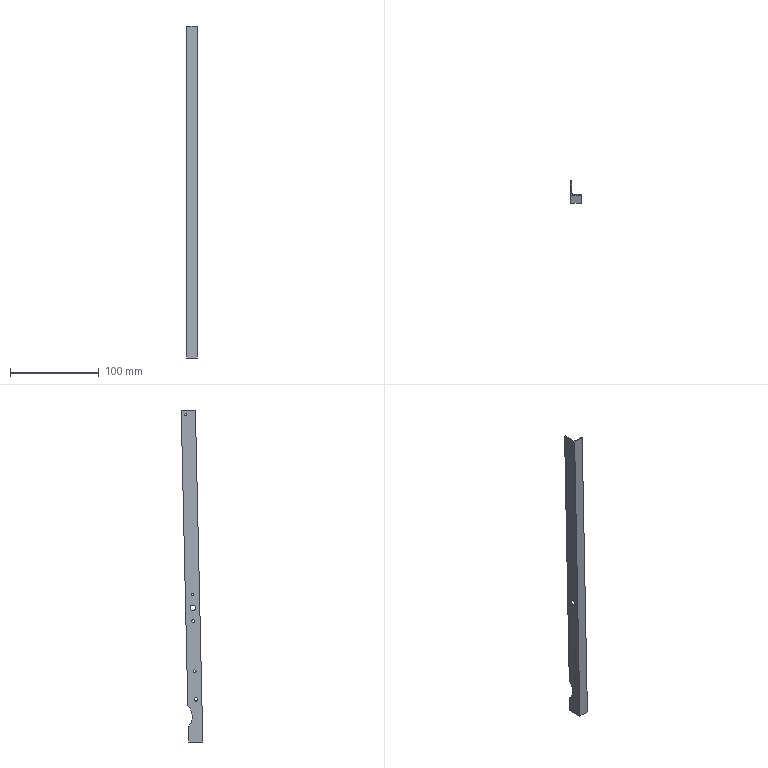Part | SolidWorks | features BaseBody 1 | 1 solid | 25 faces | box 12 x 24.318 x 374.05 mm | volume 11925 mm3 | cylinder 13 | plane 11 | spline 1 | commonest cylinder face diameters 3.2 x6 2.4 x2 4 x2 6.35 x2 36 x1
STEP:
#1=CARTESIAN_POINT('',(186.7,-128.619,106.65));
#2=VERTEX_POINT('',#1);
#3=CARTESIAN_POINT('',(186.7,-128.619,103.45));
#4=VERTEX_POINT('',#3);
#5=CARTESIAN_POINT('',(186.7,-128.619,105.05));
#6=DIRECTION('',(1.,0.,0.));
#7=DIRECTION('',(0.,0.,1.));
#8=AXIS2_PLACEMENT_3D('',#5,#6,#7);
#9=CIRCLE('',#8,1.6);
#10=EDGE_CURVE('',#2,#4,#9,.T.);
#11=ORIENTED_EDGE('',*,*,#10,.T.);
#12=CARTESIAN_POINT('',(185.5,-128.619,103.45));
#13=VERTEX_POINT('',#12);
#14=CARTESIAN_POINT('',(186.7,-128.619,103.45));
#15=DIRECTION('',(-1.,0.,0.));
#16=VECTOR('',#15,1000.);
#17=LINE('',#14,#16);
#18=EDGE_CURVE('',#4,#13,#17,.T.);
#19=ORIENTED_EDGE('',*,*,#18,.T.);
#20=CARTESIAN_POINT('',(185.5,-128.619,106.65));
#21=VERTEX_POINT('',#20);
#22=CARTESIAN_POINT('',(185.5,-128.619,105.05));
#23=DIRECTION('',(-1.,0.,0.));
#24=DIRECTION('',(0.,0.,1.));
#25=AXIS2_PLACEMENT_3D('',#22,#23,#24);
#26=CIRCLE('',#25,1.6);
#27=EDGE_CURVE('',#13,#21,#26,.T.);
#28=ORIENTED_EDGE('',*,*,#27,.T.);
#29=CARTESIAN_POINT('',(186.7,-128.619,106.65));
#30=DIRECTION('',(-1.,0.,0.));
#31=VECTOR('',#30,1000.);
#32=LINE('',#29,#31);
#33=EDGE_CURVE('',#2,#21,#32,.T.);
#34=ORIENTED_EDGE('',*,*,#33,.F.);
#35=EDGE_LOOP('',(#11,#19,#28,#34));
#36=FACE_OUTER_BOUND('',#35,.T.);
#37=CARTESIAN_POINT('',(186.7,-128.619,105.05));
#38=DIRECTION('',(-1.,0.,0.));
#39=DIRECTION('',(0.,0.,1.));
#40=AXIS2_PLACEMENT_3D('',#37,#38,#39);
#41=CYLINDRICAL_SURFACE('',#40,1.6);
#42=ADVANCED_FACE('',(#36),#41,.F.);
#43=CARTESIAN_POINT('',(185.5,-130.,71.45));
#44=VERTEX_POINT('',#43);
#45=CARTESIAN_POINT('',(185.5,-130.,75.45));
#46=VERTEX_POINT('',#45);
#47=CARTESIAN_POINT('',(185.5,-130.,73.45));
#48=DIRECTION('',(-1.,0.,0.));
#49=DIRECTION('',(0.,0.,-1.));
#50=AXIS2_PLACEMENT_3D('',#47,#48,#49);
#51=CIRCLE('',#50,2.);
#52=EDGE_CURVE('',#44,#46,#51,.T.);
#53=ORIENTED_EDGE('',*,*,#52,.T.);
#54=CARTESIAN_POINT('',(186.7,-130.,75.45));
#55=VERTEX_POINT('',#54);
#56=CARTESIAN_POINT('',(185.5,-130.,75.45));
#57=DIRECTION('',(1.,0.,0.));
#58=VECTOR('',#57,1000.);
#59=LINE('',#56,#58);
#60=EDGE_CURVE('',#46,#55,#59,.T.);
#61=ORIENTED_EDGE('',*,*,#60,.T.);
#62=CARTESIAN_POINT('',(186.7,-130.,71.45));
#63=VERTEX_POINT('',#62);
#64=CARTESIAN_POINT('',(186.7,-130.,73.45));
#65=DIRECTION('',(1.,0.,0.));
#66=DIRECTION('',(0.,0.,-1.));
#67=AXIS2_PLACEMENT_3D('',#64,#65,#66);
#68=CIRCLE('',#67,2.);
#69=EDGE_CURVE('',#55,#63,#68,.T.);
#70=ORIENTED_EDGE('',*,*,#69,.T.);
#71=CARTESIAN_POINT('',(185.5,-130.,71.45));
#72=DIRECTION('',(1.,0.,0.));
#73=VECTOR('',#72,1000.);
#74=LINE('',#71,#73);
#75=EDGE_CURVE('',#44,#63,#74,.T.);
#76=ORIENTED_EDGE('',*,*,#75,.F.);
#77=EDGE_LOOP('',(#53,#61,#70,#76));
#78=FACE_OUTER_BOUND('',#77,.T.);
#79=CARTESIAN_POINT('',(185.5,-130.,73.45));
#80=DIRECTION('',(1.,0.,0.));
#81=DIRECTION('',(0.,0.,-1.));
#82=AXIS2_PLACEMENT_3D('',#79,#80,#81);
#83=CYLINDRICAL_SURFACE('',#82,2.);
#84=ADVANCED_FACE('',(#78),#83,.F.);
#85=CARTESIAN_POINT('',(185.5,-118.471,392.8));
#86=VERTEX_POINT('',#85);
#87=CARTESIAN_POINT('',(185.5,-118.471,395.2));
#88=VERTEX_POINT('',#87);
#89=CARTESIAN_POINT('',(185.5,-118.471,394.));
#90=DIRECTION('',(-1.,0.,0.));
#91=DIRECTION('',(0.,0.,-1.));
#92=AXIS2_PLACEMENT_3D('',#89,#90,#91);
#93=CIRCLE('',#92,1.2);
#94=EDGE_CURVE('',#86,#88,#93,.T.);
#95=ORIENTED_EDGE('',*,*,#94,.T.);
#96=CARTESIAN_POINT('',(186.7,-118.471,395.2));
#97=VERTEX_POINT('',#96);
#98=CARTESIAN_POINT('',(185.5,-118.471,395.2));
#99=DIRECTION('',(1.,0.,0.));
#100=VECTOR('',#99,1000.);
#101=LINE('',#98,#100);
#102=EDGE_CURVE('',#88,#97,#101,.T.);
#103=ORIENTED_EDGE('',*,*,#102,.T.);
#104=CARTESIAN_POINT('',(186.7,-118.471,392.8));
#105=VERTEX_POINT('',#104);
#106=CARTESIAN_POINT('',(186.7,-118.471,394.));
#107=DIRECTION('',(1.,0.,0.));
#108=DIRECTION('',(0.,0.,-1.));
#109=AXIS2_PLACEMENT_3D('',#106,#107,#108);
#110=CIRCLE('',#109,1.2);
#111=EDGE_CURVE('',#97,#105,#110,.T.);
#112=ORIENTED_EDGE('',*,*,#111,.T.);
#113=CARTESIAN_POINT('',(185.5,-118.471,392.8));
#114=DIRECTION('',(1.,0.,0.));
#115=VECTOR('',#114,1000.);
#116=LINE('',#113,#115);
#117=EDGE_CURVE('',#86,#105,#116,.T.);
#118=ORIENTED_EDGE('',*,*,#117,.F.);
#119=EDGE_LOOP('',(#95,#103,#112,#118));
#120=FACE_OUTER_BOUND('',#119,.T.);
#121=CARTESIAN_POINT('',(185.5,-118.471,394.));
#122=DIRECTION('',(1.,0.,0.));
#123=DIRECTION('',(0.,0.,-1.));
#124=AXIS2_PLACEMENT_3D('',#121,#122,#123);
#125=CYLINDRICAL_SURFACE('',#124,1.2);
#126=ADVANCED_FACE('',(#120),#125,.F.);
#127=CARTESIAN_POINT('',(186.7,-126.564,179.8));
#128=VERTEX_POINT('',#127);
#129=CARTESIAN_POINT('',(186.7,-126.564,173.45));
#130=VERTEX_POINT('',#129);
#131=CARTESIAN_POINT('',(186.7,-126.564,176.625));
#132=DIRECTION('',(1.,0.,0.));
#133=DIRECTION('',(0.,0.,1.));
#134=AXIS2_PLACEMENT_3D('',#131,#132,#133);
#135=CIRCLE('',#134,3.175);
#136=EDGE_CURVE('',#128,#130,#135,.T.);
#137=ORIENTED_EDGE('',*,*,#136,.T.);
#138=CARTESIAN_POINT('',(185.5,-126.564,173.45));
#139=VERTEX_POINT('',#138);
#140=CARTESIAN_POINT('',(186.7,-126.564,173.45));
#141=DIRECTION('',(-1.,0.,0.));
#142=VECTOR('',#141,1000.);
#143=LINE('',#140,#142);
#144=EDGE_CURVE('',#130,#139,#143,.T.);
#145=ORIENTED_EDGE('',*,*,#144,.T.);
#146=CARTESIAN_POINT('',(185.5,-126.564,179.8));
#147=VERTEX_POINT('',#146);
#148=CARTESIAN_POINT('',(185.5,-126.564,176.625));
#149=DIRECTION('',(-1.,0.,0.));
#150=DIRECTION('',(0.,0.,1.));
#151=AXIS2_PLACEMENT_3D('',#148,#149,#150);
#152=CIRCLE('',#151,3.175);
#153=EDGE_CURVE('',#139,#147,#152,.T.);
#154=ORIENTED_EDGE('',*,*,#153,.T.);
#155=CARTESIAN_POINT('',(186.7,-126.564,179.8));
#156=DIRECTION('',(-1.,0.,0.));
#157=VECTOR('',#156,1000.);
#158=LINE('',#155,#157);
#159=EDGE_CURVE('',#128,#147,#158,.T.);
#160=ORIENTED_EDGE('',*,*,#159,.F.);
#161=EDGE_LOOP('',(#137,#145,#154,#160));
#162=FACE_OUTER_BOUND('',#161,.T.);
#163=CARTESIAN_POINT('',(186.7,-126.564,176.625));
#164=DIRECTION('',(-1.,0.,0.));
#165=DIRECTION('',(0.,0.,1.));
#166=AXIS2_PLACEMENT_3D('',#163,#164,#165);
#167=CYLINDRICAL_SURFACE('',#166,3.175);
#168=ADVANCED_FACE('',(#162),#167,.F.);
#169=CARTESIAN_POINT('',(186.7,-126.905,163.229));
#170=VERTEX_POINT('',#169);
#171=CARTESIAN_POINT('',(186.7,-126.905,160.029));
#172=VERTEX_POINT('',#171);
#173=CARTESIAN_POINT('',(186.7,-126.905,161.629));
#174=DIRECTION('',(1.,0.,0.));
#175=DIRECTION('',(0.,0.,1.));
#176=AXIS2_PLACEMENT_3D('',#173,#174,#175);
#177=CIRCLE('',#176,1.6);
#178=EDGE_CURVE('',#170,#172,#177,.T.);
#179=ORIENTED_EDGE('',*,*,#178,.T.);
#180=CARTESIAN_POINT('',(185.5,-126.905,160.029));
#181=VERTEX_POINT('',#180);
#182=CARTESIAN_POINT('',(186.7,-126.905,160.029));
#183=DIRECTION('',(-1.,0.,0.));
#184=VECTOR('',#183,1000.);
#185=LINE('',#182,#184);
#186=EDGE_CURVE('',#172,#181,#185,.T.);
#187=ORIENTED_EDGE('',*,*,#186,.T.);
#188=CARTESIAN_POINT('',(185.5,-126.905,163.229));
#189=VERTEX_POINT('',#188);
#190=CARTESIAN_POINT('',(185.5,-126.905,161.629));
#191=DIRECTION('',(-1.,0.,0.));
#192=DIRECTION('',(0.,0.,1.));
#193=AXIS2_PLACEMENT_3D('',#190,#191,#192);
#194=CIRCLE('',#193,1.6);
#195=EDGE_CURVE('',#181,#189,#194,.T.);
#196=ORIENTED_EDGE('',*,*,#195,.T.);
#197=CARTESIAN_POINT('',(186.7,-126.905,163.229));
#198=DIRECTION('',(-1.,0.,0.));
#199=VECTOR('',#198,1000.);
#200=LINE('',#197,#199);
#201=EDGE_CURVE('',#170,#189,#200,.T.);
#202=ORIENTED_EDGE('',*,*,#201,.F.);
#203=EDGE_LOOP('',(#179,#187,#196,#202));
#204=FACE_OUTER_BOUND('',#203,.T.);
#205=CARTESIAN_POINT('',(186.7,-126.905,161.629));
#206=DIRECTION('',(-1.,0.,0.));
#207=DIRECTION('',(0.,0.,1.));
#208=AXIS2_PLACEMENT_3D('',#205,#206,#207);
#209=CYLINDRICAL_SURFACE('',#208,1.6);
#210=ADVANCED_FACE('',(#204),#209,.F.);
#211=CARTESIAN_POINT('',(186.7,-126.223,193.221));
#212=VERTEX_POINT('',#211);
#213=CARTESIAN_POINT('',(186.7,-126.223,190.021));
#214=VERTEX_POINT('',#213);
#215=CARTESIAN_POINT('',(186.7,-126.223,191.621));
#216=DIRECTION('',(1.,0.,0.));
#217=DIRECTION('',(0.,0.,1.));
#218=AXIS2_PLACEMENT_3D('',#215,#216,#217);
#219=CIRCLE('',#218,1.6);
#220=EDGE_CURVE('',#212,#214,#219,.T.);
#221=ORIENTED_EDGE('',*,*,#220,.T.);
#222=CARTESIAN_POINT('',(185.5,-126.223,190.021));
#223=VERTEX_POINT('',#222);
#224=CARTESIAN_POINT('',(186.7,-126.223,190.021));
#225=DIRECTION('',(-1.,0.,0.));
#226=VECTOR('',#225,1000.);
#227=LINE('',#224,#226);
#228=EDGE_CURVE('',#214,#223,#227,.T.);
#229=ORIENTED_EDGE('',*,*,#228,.T.);
#230=CARTESIAN_POINT('',(185.5,-126.223,193.221));
#231=VERTEX_POINT('',#230);
#232=CARTESIAN_POINT('',(185.5,-126.223,191.621));
#233=DIRECTION('',(-1.,0.,0.));
#234=DIRECTION('',(0.,0.,1.));
#235=AXIS2_PLACEMENT_3D('',#232,#233,#234);
#236=CIRCLE('',#235,1.6);
#237=EDGE_CURVE('',#223,#231,#236,.T.);
#238=ORIENTED_EDGE('',*,*,#237,.T.);
#239=CARTESIAN_POINT('',(186.7,-126.223,193.221));
#240=DIRECTION('',(-1.,0.,0.));
#241=VECTOR('',#240,1000.);
#242=LINE('',#239,#241);
#243=EDGE_CURVE('',#212,#231,#242,.T.);
#244=ORIENTED_EDGE('',*,*,#243,.F.);
#245=EDGE_LOOP('',(#221,#229,#238,#244));
#246=FACE_OUTER_BOUND('',#245,.T.);
#247=CARTESIAN_POINT('',(186.7,-126.223,191.621));
#248=DIRECTION('',(-1.,0.,0.));
#249=DIRECTION('',(0.,0.,1.));
#250=AXIS2_PLACEMENT_3D('',#247,#248,#249);
#251=CYLINDRICAL_SURFACE('',#250,1.6);
#252=ADVANCED_FACE('',(#246),#251,.F.);
#253=ORIENTED_EDGE('',*,*,#18,.F.);
#254=CARTESIAN_POINT('',(186.7,-128.619,105.05));
#255=DIRECTION('',(1.,0.,0.));
#256=DIRECTION('',(0.,0.,1.));
#257=AXIS2_PLACEMENT_3D('',#254,#255,#256);
#258=CIRCLE('',#257,1.6);
#259=EDGE_CURVE('',#4,#2,#258,.T.);
#260=ORIENTED_EDGE('',*,*,#259,.T.);
#261=ORIENTED_EDGE('',*,*,#33,.T.);
#262=CARTESIAN_POINT('',(185.5,-128.619,105.05));
#263=DIRECTION('',(-1.,0.,0.));
#264=DIRECTION('',(0.,0.,1.));
#265=AXIS2_PLACEMENT_3D('',#262,#263,#264);
#266=CIRCLE('',#265,1.6);
#267=EDGE_CURVE('',#21,#13,#266,.T.);
#268=ORIENTED_EDGE('',*,*,#267,.T.);
#269=EDGE_LOOP('',(#253,#260,#261,#268));
#270=FACE_OUTER_BOUND('',#269,.T.);
#271=CARTESIAN_POINT('',(186.7,-128.619,105.05));
#272=DIRECTION('',(-1.,0.,0.));
#273=DIRECTION('',(0.,0.,1.));
#274=AXIS2_PLACEMENT_3D('',#271,#272,#273);
#275=CYLINDRICAL_SURFACE('',#274,1.6);
#276=ADVANCED_FACE('',(#270),#275,.F.);
#277=ORIENTED_EDGE('',*,*,#52,.F.);
#278=CARTESIAN_POINT('',(185.5,-130.,73.45));
#279=DIRECTION('',(-1.,0.,0.));
#280=DIRECTION('',(0.,0.,-1.));
#281=AXIS2_PLACEMENT_3D('',#278,#279,#280);
#282=CIRCLE('',#281,2.);
#283=EDGE_CURVE('',#46,#44,#282,.T.);
#284=ORIENTED_EDGE('',*,*,#283,.F.);
#285=EDGE_LOOP('',(#277,#284));
#286=FACE_BOUND('',#285,.T.);
#287=ORIENTED_EDGE('',*,*,#94,.F.);
#288=CARTESIAN_POINT('',(185.5,-118.471,394.));
#289=DIRECTION('',(-1.,0.,0.));
#290=DIRECTION('',(0.,0.,-1.));
#291=AXIS2_PLACEMENT_3D('',#288,#289,#290);
#292=CIRCLE('',#291,1.2);
#293=EDGE_CURVE('',#88,#86,#292,.T.);
#294=ORIENTED_EDGE('',*,*,#293,.F.);
#295=EDGE_LOOP('',(#287,#294));
#296=FACE_BOUND('',#295,.T.);
#297=CARTESIAN_POINT('',(185.5,-126.564,176.625));
#298=DIRECTION('',(-1.,0.,0.));
#299=DIRECTION('',(0.,0.,1.));
#300=AXIS2_PLACEMENT_3D('',#297,#298,#299);
#301=CIRCLE('',#300,3.175);
#302=EDGE_CURVE('',#147,#139,#301,.T.);
#303=ORIENTED_EDGE('',*,*,#302,.F.);
#304=ORIENTED_EDGE('',*,*,#153,.F.);
#305=EDGE_LOOP('',(#303,#304));
#306=FACE_BOUND('',#305,.T.);
#307=CARTESIAN_POINT('',(185.5,-126.905,161.629));
#308=DIRECTION('',(-1.,0.,0.));
#309=DIRECTION('',(0.,0.,1.));
#310=AXIS2_PLACEMENT_3D('',#307,#308,#309);
#311=CIRCLE('',#310,1.6);
#312=EDGE_CURVE('',#189,#181,#311,.T.);
#313=ORIENTED_EDGE('',*,*,#312,.F.);
#314=ORIENTED_EDGE('',*,*,#195,.F.);
#315=EDGE_LOOP('',(#313,#314));
#316=FACE_BOUND('',#315,.T.);
#317=CARTESIAN_POINT('',(185.5,-126.223,191.621));
#318=DIRECTION('',(-1.,0.,0.));
#319=DIRECTION('',(0.,0.,1.));
#320=AXIS2_PLACEMENT_3D('',#317,#318,#319);
#321=CIRCLE('',#320,1.6);
#322=EDGE_CURVE('',#231,#223,#321,.T.);
#323=ORIENTED_EDGE('',*,*,#322,.F.);
#324=ORIENTED_EDGE('',*,*,#237,.F.);
#325=EDGE_LOOP('',(#323,#324));
#326=FACE_BOUND('',#325,.T.);
#327=ORIENTED_EDGE('',*,*,#267,.F.);
#328=ORIENTED_EDGE('',*,*,#27,.F.);
#329=EDGE_LOOP('',(#327,#328));
#330=FACE_BOUND('',#329,.T.);
#331=CARTESIAN_POINT('',(185.5,-121.435,42.365));
#332=VERTEX_POINT('',#331);
#333=CARTESIAN_POINT('',(185.5,-121.619,42.181));
#334=VERTEX_POINT('',#333);
#335=CARTESIAN_POINT('',(185.5,-121.619,42.181));
#336=DIRECTION('',(0.,-0.7071,-0.7071));
#337=VECTOR('',#336,1000.);
#338=LINE('',#335,#337);
#339=EDGE_CURVE('',#332,#334,#338,.T.);
#340=ORIENTED_EDGE('',*,*,#339,.F.);
#341=CARTESIAN_POINT('',(185.5,-121.811,25.45));
#342=VERTEX_POINT('',#341);
#343=CARTESIAN_POINT('',(185.5,-121.435,42.365));
#344=DIRECTION('',(0.,0.02223,0.9998));
#345=VECTOR('',#344,1000.);
#346=LINE('',#343,#345);
#347=EDGE_CURVE('',#342,#332,#346,.T.);
#348=ORIENTED_EDGE('',*,*,#347,.F.);
#349=CARTESIAN_POINT('',(185.5,-137.811,25.45));
#350=VERTEX_POINT('',#349);
#351=CARTESIAN_POINT('',(185.5,-125.652,25.45));
#352=DIRECTION('',(0.,1.,0.));
#353=VECTOR('',#352,1000.);
#354=LINE('',#351,#353);
#355=EDGE_CURVE('',#350,#342,#354,.T.);
#356=ORIENTED_EDGE('',*,*,#355,.F.);
#357=CARTESIAN_POINT('',(185.5,-129.494,399.5));
#358=VERTEX_POINT('',#357);
#359=CARTESIAN_POINT('',(185.5,-137.811,25.45));
#360=DIRECTION('',(0.,-0.02223,-0.9998));
#361=VECTOR('',#360,1000.);
#362=LINE('',#359,#361);
#363=EDGE_CURVE('',#358,#350,#362,.T.);
#364=ORIENTED_EDGE('',*,*,#363,.F.);
#365=CARTESIAN_POINT('',(185.5,-113.494,399.5));
#366=VERTEX_POINT('',#365);
#367=CARTESIAN_POINT('',(185.5,-125.652,399.5));
#368=DIRECTION('',(0.,-1.,0.));
#369=VECTOR('',#368,1000.);
#370=LINE('',#367,#369);
#371=EDGE_CURVE('',#366,#358,#370,.T.);
#372=ORIENTED_EDGE('',*,*,#371,.F.);
#373=CARTESIAN_POINT('',(185.5,-120.906,66.145));
#374=VERTEX_POINT('',#373);
#375=CARTESIAN_POINT('',(185.5,-113.494,399.5));
#376=DIRECTION('',(0.,0.02223,0.9998));
#377=VECTOR('',#376,1000.);
#378=LINE('',#375,#377);
#379=EDGE_CURVE('',#374,#366,#378,.T.);
#380=ORIENTED_EDGE('',*,*,#379,.F.);
#381=CARTESIAN_POINT('',(185.5,-121.07,66.326));
#382=VERTEX_POINT('',#381);
#383=CARTESIAN_POINT('',(185.5,-120.906,66.145));
#384=DIRECTION('',(0.,0.6717,-0.7409));
#385=VECTOR('',#384,1000.);
#386=LINE('',#383,#385);
#387=EDGE_CURVE('',#382,#374,#386,.T.);
#388=ORIENTED_EDGE('',*,*,#387,.F.);
#389=CARTESIAN_POINT('',(185.5,-108.,53.95));
#390=DIRECTION('',(-1.,0.,0.));
#391=DIRECTION('',(0.,0.,1.));
#392=AXIS2_PLACEMENT_3D('',#389,#390,#391);
#393=CIRCLE('',#392,18.);
#394=EDGE_CURVE('',#334,#382,#393,.T.);
#395=ORIENTED_EDGE('',*,*,#394,.F.);
#396=EDGE_LOOP('',(#340,#348,#356,#364,#372,#380,#388,#395));
#397=FACE_OUTER_BOUND('',#396,.T.);
#398=CARTESIAN_POINT('',(185.5,-137.957,399.5));
#399=DIRECTION('',(1.,0.,0.));
#400=DIRECTION('',(0.,0.,-1.));
#401=AXIS2_PLACEMENT_3D('',#398,#399,#400);
#402=PLANE('',#401);
#403=ADVANCED_FACE('',(#286,#296,#306,#316,#326,#330,#397),#402,.F.);
#404=CARTESIAN_POINT('',(186.7,-130.,73.45));
#405=DIRECTION('',(1.,0.,0.));
#406=DIRECTION('',(0.,0.,-1.));
#407=AXIS2_PLACEMENT_3D('',#404,#405,#406);
#408=CIRCLE('',#407,2.);
#409=EDGE_CURVE('',#63,#55,#408,.T.);
#410=ORIENTED_EDGE('',*,*,#409,.F.);
#411=ORIENTED_EDGE('',*,*,#69,.F.);
#412=EDGE_LOOP('',(#410,#411));
#413=FACE_BOUND('',#412,.T.);
#414=CARTESIAN_POINT('',(186.7,-118.471,394.));
#415=DIRECTION('',(1.,0.,0.));
#416=DIRECTION('',(0.,0.,-1.));
#417=AXIS2_PLACEMENT_3D('',#414,#415,#416);
#418=CIRCLE('',#417,1.2);
#419=EDGE_CURVE('',#105,#97,#418,.T.);
#420=ORIENTED_EDGE('',*,*,#419,.F.);
#421=ORIENTED_EDGE('',*,*,#111,.F.);
#422=EDGE_LOOP('',(#420,#421));
#423=FACE_BOUND('',#422,.T.);
#424=ORIENTED_EDGE('',*,*,#136,.F.);
#425=CARTESIAN_POINT('',(186.7,-126.564,176.625));
#426=DIRECTION('',(1.,0.,0.));
#427=DIRECTION('',(0.,0.,1.));
#428=AXIS2_PLACEMENT_3D('',#425,#426,#427);
#429=CIRCLE('',#428,3.175);
#430=EDGE_CURVE('',#130,#128,#429,.T.);
#431=ORIENTED_EDGE('',*,*,#430,.F.);
#432=EDGE_LOOP('',(#424,#431));
#433=FACE_BOUND('',#432,.T.);
#434=ORIENTED_EDGE('',*,*,#178,.F.);
#435=CARTESIAN_POINT('',(186.7,-126.905,161.629));
#436=DIRECTION('',(1.,0.,0.));
#437=DIRECTION('',(0.,0.,1.));
#438=AXIS2_PLACEMENT_3D('',#435,#436,#437);
#439=CIRCLE('',#438,1.6);
#440=EDGE_CURVE('',#172,#170,#439,.T.);
#441=ORIENTED_EDGE('',*,*,#440,.F.);
#442=EDGE_LOOP('',(#434,#441));
#443=FACE_BOUND('',#442,.T.);
#444=ORIENTED_EDGE('',*,*,#220,.F.);
#445=CARTESIAN_POINT('',(186.7,-126.223,191.621));
#446=DIRECTION('',(1.,0.,0.));
#447=DIRECTION('',(0.,0.,1.));
#448=AXIS2_PLACEMENT_3D('',#445,#446,#447);
#449=CIRCLE('',#448,1.6);
#450=EDGE_CURVE('',#214,#212,#449,.T.);
#451=ORIENTED_EDGE('',*,*,#450,.F.);
#452=EDGE_LOOP('',(#444,#451));
#453=FACE_BOUND('',#452,.T.);
#454=ORIENTED_EDGE('',*,*,#10,.F.);
#455=ORIENTED_EDGE('',*,*,#259,.F.);
#456=EDGE_LOOP('',(#454,#455));
#457=FACE_BOUND('',#456,.T.);
#458=CARTESIAN_POINT('',(186.7,-121.619,42.181));
#459=VERTEX_POINT('',#458);
#460=CARTESIAN_POINT('',(186.7,-121.435,42.365));
#461=VERTEX_POINT('',#460);
#462=CARTESIAN_POINT('',(186.7,-121.619,42.181));
#463=DIRECTION('',(0.,0.7071,0.7071));
#464=VECTOR('',#463,1000.);
#465=LINE('',#462,#464);
#466=EDGE_CURVE('',#459,#461,#465,.T.);
#467=ORIENTED_EDGE('',*,*,#466,.F.);
#468=CARTESIAN_POINT('',(186.7,-121.07,66.326));
#469=VERTEX_POINT('',#468);
#470=CARTESIAN_POINT('',(186.7,-108.,53.95));
#471=DIRECTION('',(1.,0.,0.));
#472=DIRECTION('',(0.,0.,1.));
#473=AXIS2_PLACEMENT_3D('',#470,#471,#472);
#474=CIRCLE('',#473,18.);
#475=EDGE_CURVE('',#469,#459,#474,.T.);
#476=ORIENTED_EDGE('',*,*,#475,.F.);
#477=CARTESIAN_POINT('',(186.7,-120.906,66.145));
#478=VERTEX_POINT('',#477);
#479=CARTESIAN_POINT('',(186.7,-120.906,66.145));
#480=DIRECTION('',(0.,-0.6717,0.7409));
#481=VECTOR('',#480,1000.);
#482=LINE('',#479,#481);
#483=EDGE_CURVE('',#478,#469,#482,.T.);
#484=ORIENTED_EDGE('',*,*,#483,.F.);
#485=CARTESIAN_POINT('',(186.7,-113.494,399.5));
#486=VERTEX_POINT('',#485);
#487=CARTESIAN_POINT('',(186.7,-113.494,399.5));
#488=DIRECTION('',(0.,-0.02223,-0.9998));
#489=VECTOR('',#488,1000.);
#490=LINE('',#487,#489);
#491=EDGE_CURVE('',#486,#478,#490,.T.);
#492=ORIENTED_EDGE('',*,*,#491,.F.);
#493=CARTESIAN_POINT('',(186.7,-127.294,399.5));
#494=VERTEX_POINT('',#493);
#495=CARTESIAN_POINT('',(186.7,-124.552,399.5));
#496=DIRECTION('',(0.,1.,0.));
#497=VECTOR('',#496,1000.);
#498=LINE('',#495,#497);
#499=EDGE_CURVE('',#494,#486,#498,.T.);
#500=ORIENTED_EDGE('',*,*,#499,.F.);
#501=CARTESIAN_POINT('',(186.7,-135.611,25.45));
#502=VERTEX_POINT('',#501);
#503=CARTESIAN_POINT('',(186.7,-127.294,399.5));
#504=DIRECTION('',(0.,0.02223,0.9998));
#505=VECTOR('',#504,1000.);
#506=LINE('',#503,#505);
#507=EDGE_CURVE('',#502,#494,#506,.T.);
#508=ORIENTED_EDGE('',*,*,#507,.F.);
#509=CARTESIAN_POINT('',(186.7,-121.811,25.45));
#510=VERTEX_POINT('',#509);
#511=CARTESIAN_POINT('',(186.7,-124.552,25.45));
#512=DIRECTION('',(0.,-1.,0.));
#513=VECTOR('',#512,1000.);
#514=LINE('',#511,#513);
#515=EDGE_CURVE('',#510,#502,#514,.T.);
#516=ORIENTED_EDGE('',*,*,#515,.F.);
#517=CARTESIAN_POINT('',(186.7,-121.435,42.365));
#518=DIRECTION('',(0.,-0.02223,-0.9998));
#519=VECTOR('',#518,1000.);
#520=LINE('',#517,#519);
#521=EDGE_CURVE('',#461,#510,#520,.T.);
#522=ORIENTED_EDGE('',*,*,#521,.F.);
#523=EDGE_LOOP('',(#467,#476,#484,#492,#500,#508,#516,#522));
#524=FACE_OUTER_BOUND('',#523,.T.);
#525=CARTESIAN_POINT('',(186.7,-135.744,25.45));
#526=DIRECTION('',(-1.,0.,0.));
#527=DIRECTION('',(0.,0.,1.));
#528=AXIS2_PLACEMENT_3D('',#525,#526,#527);
#529=PLANE('',#528);
#530=ADVANCED_FACE('',(#413,#423,#433,#443,#453,#457,#524),#529,.F.);
#531=ORIENTED_EDGE('',*,*,#60,.F.);
#532=ORIENTED_EDGE('',*,*,#283,.T.);
#533=ORIENTED_EDGE('',*,*,#75,.T.);
#534=ORIENTED_EDGE('',*,*,#409,.T.);
#535=EDGE_LOOP('',(#531,#532,#533,#534));
#536=FACE_OUTER_BOUND('',#535,.T.);
#537=CARTESIAN_POINT('',(185.5,-130.,73.45));
#538=DIRECTION('',(1.,0.,0.));
#539=DIRECTION('',(0.,0.,-1.));
#540=AXIS2_PLACEMENT_3D('',#537,#538,#539);
#541=CYLINDRICAL_SURFACE('',#540,2.);
#542=ADVANCED_FACE('',(#536),#541,.F.);
#543=ORIENTED_EDGE('',*,*,#102,.F.);
#544=ORIENTED_EDGE('',*,*,#293,.T.);
#545=ORIENTED_EDGE('',*,*,#117,.T.);
#546=ORIENTED_EDGE('',*,*,#419,.T.);
#547=EDGE_LOOP('',(#543,#544,#545,#546));
#548=FACE_OUTER_BOUND('',#547,.T.);
#549=CARTESIAN_POINT('',(185.5,-118.471,394.));
#550=DIRECTION('',(1.,0.,0.));
#551=DIRECTION('',(0.,0.,-1.));
#552=AXIS2_PLACEMENT_3D('',#549,#550,#551);
#553=CYLINDRICAL_SURFACE('',#552,1.2);
#554=ADVANCED_FACE('',(#548),#553,.F.);
#555=ORIENTED_EDGE('',*,*,#144,.F.);
#556=ORIENTED_EDGE('',*,*,#430,.T.);
#557=ORIENTED_EDGE('',*,*,#159,.T.);
#558=ORIENTED_EDGE('',*,*,#302,.T.);
#559=EDGE_LOOP('',(#555,#556,#557,#558));
#560=FACE_OUTER_BOUND('',#559,.T.);
#561=CARTESIAN_POINT('',(186.7,-126.564,176.625));
#562=DIRECTION('',(-1.,0.,0.));
#563=DIRECTION('',(0.,0.,1.));
#564=AXIS2_PLACEMENT_3D('',#561,#562,#563);
#565=CYLINDRICAL_SURFACE('',#564,3.175);
#566=ADVANCED_FACE('',(#560),#565,.F.);
#567=ORIENTED_EDGE('',*,*,#186,.F.);
#568=ORIENTED_EDGE('',*,*,#440,.T.);
#569=ORIENTED_EDGE('',*,*,#201,.T.);
#570=ORIENTED_EDGE('',*,*,#312,.T.);
#571=EDGE_LOOP('',(#567,#568,#569,#570));
#572=FACE_OUTER_BOUND('',#571,.T.);
#573=CARTESIAN_POINT('',(186.7,-126.905,161.629));
#574=DIRECTION('',(-1.,0.,0.));
#575=DIRECTION('',(0.,0.,1.));
#576=AXIS2_PLACEMENT_3D('',#573,#574,#575);
#577=CYLINDRICAL_SURFACE('',#576,1.6);
#578=ADVANCED_FACE('',(#572),#577,.F.);
#579=ORIENTED_EDGE('',*,*,#228,.F.);
#580=ORIENTED_EDGE('',*,*,#450,.T.);
#581=ORIENTED_EDGE('',*,*,#243,.T.);
#582=ORIENTED_EDGE('',*,*,#322,.T.);
#583=EDGE_LOOP('',(#579,#580,#581,#582));
#584=FACE_OUTER_BOUND('',#583,.T.);
#585=CARTESIAN_POINT('',(186.7,-126.223,191.621));
#586=DIRECTION('',(-1.,0.,0.));
#587=DIRECTION('',(0.,0.,1.));
#588=AXIS2_PLACEMENT_3D('',#585,#586,#587);
#589=CYLINDRICAL_SURFACE('',#588,1.6);
#590=ADVANCED_FACE('',(#584),#589,.F.);
#591=CARTESIAN_POINT('',(186.1,-121.07,66.326));
#592=DIRECTION('',(1.,0.,0.));
#593=VECTOR('',#592,1000.);
#594=LINE('',#591,#593);
#595=EDGE_CURVE('',#382,#469,#594,.T.);
#596=ORIENTED_EDGE('',*,*,#595,.T.);
#597=ORIENTED_EDGE('',*,*,#475,.T.);
#598=CARTESIAN_POINT('',(186.1,-121.619,42.181));
#599=DIRECTION('',(-1.,0.,0.));
#600=VECTOR('',#599,1000.);
#601=LINE('',#598,#600);
#602=EDGE_CURVE('',#459,#334,#601,.T.);
#603=ORIENTED_EDGE('',*,*,#602,.T.);
#604=ORIENTED_EDGE('',*,*,#394,.T.);
#605=EDGE_LOOP('',(#596,#597,#603,#604));
#606=FACE_OUTER_BOUND('',#605,.T.);
#607=CARTESIAN_POINT('',(186.7,-108.,53.95));
#608=DIRECTION('',(-1.,0.,0.));
#609=DIRECTION('',(0.,0.,1.));
#610=AXIS2_PLACEMENT_3D('',#607,#608,#609);
#611=CYLINDRICAL_SURFACE('',#610,18.);
#612=ADVANCED_FACE('',(#606),#611,.F.);
#613=ORIENTED_EDGE('',*,*,#602,.F.);
#614=ORIENTED_EDGE('',*,*,#466,.T.);
#615=CARTESIAN_POINT('',(186.1,-121.435,42.365));
#616=DIRECTION('',(1.,0.,0.));
#617=VECTOR('',#616,1000.);
#618=LINE('',#615,#617);
#619=EDGE_CURVE('',#332,#461,#618,.T.);
#620=ORIENTED_EDGE('',*,*,#619,.F.);
#621=ORIENTED_EDGE('',*,*,#339,.T.);
#622=EDGE_LOOP('',(#613,#614,#620,#621));
#623=FACE_OUTER_BOUND('',#622,.T.);
#624=CARTESIAN_POINT('',(185.5,-121.619,42.181));
#625=DIRECTION('',(0.,0.7071,-0.7071));
#626=DIRECTION('',(0.,0.7071,0.7071));
#627=AXIS2_PLACEMENT_3D('',#624,#625,#626);
#628=PLANE('',#627);
#629=ADVANCED_FACE('',(#623),#628,.F.);
#630=ORIENTED_EDGE('',*,*,#619,.T.);
#631=ORIENTED_EDGE('',*,*,#521,.T.);
#632=CARTESIAN_POINT('',(186.1,-121.811,25.45));
#633=DIRECTION('',(1.,0.,0.));
#634=VECTOR('',#633,1000.);
#635=LINE('',#632,#634);
#636=EDGE_CURVE('',#342,#510,#635,.T.);
#637=ORIENTED_EDGE('',*,*,#636,.F.);
#638=ORIENTED_EDGE('',*,*,#347,.T.);
#639=EDGE_LOOP('',(#630,#631,#637,#638));
#640=FACE_OUTER_BOUND('',#639,.T.);
#641=CARTESIAN_POINT('',(185.5,-121.435,42.365));
#642=DIRECTION('',(0.,-0.9998,0.02223));
#643=DIRECTION('',(0.,-0.02223,-0.9998));
#644=AXIS2_PLACEMENT_3D('',#641,#642,#643);
#645=PLANE('',#644);
#646=ADVANCED_FACE('',(#640),#645,.F.);
#647=ORIENTED_EDGE('',*,*,#515,.T.);
#648=CARTESIAN_POINT('',(187.7,-136.611,25.45));
#649=VERTEX_POINT('',#648);
#650=CARTESIAN_POINT('',(187.7,-136.611,25.45));
#651=CARTESIAN_POINT('',(187.114,-136.611,25.45));
#652=CARTESIAN_POINT('',(186.7,-136.197,25.45));
#653=CARTESIAN_POINT('',(186.7,-135.611,25.45));
#654=(BOUNDED_CURVE()B_SPLINE_CURVE(3,(#650,#651,#652,#653),.UNSPECIFIED.,.F.,.F.)B_SPLINE_CURVE_WITH_KNOTS((4,4),(0.,0.001562),.UNSPECIFIED.)CURVE()GEOMETRIC_REPRESENTATION_ITEM()RATIONAL_B_SPLINE_CURVE((1.,0.8047,0.8047,1.))REPRESENTATION_ITEM(''));
#655=EDGE_CURVE('',#649,#502,#654,.T.);
#656=ORIENTED_EDGE('',*,*,#655,.F.);
#657=CARTESIAN_POINT('',(197.5,-136.611,25.45));
#658=VERTEX_POINT('',#657);
#659=CARTESIAN_POINT('',(191.5,-136.611,25.45));
#660=DIRECTION('',(-1.,0.,0.));
#661=VECTOR('',#660,1000.);
#662=LINE('',#659,#661);
#663=EDGE_CURVE('',#658,#649,#662,.T.);
#664=ORIENTED_EDGE('',*,*,#663,.F.);
#665=CARTESIAN_POINT('',(197.5,-137.811,25.45));
#666=VERTEX_POINT('',#665);
#667=CARTESIAN_POINT('',(197.5,-133.052,25.45));
#668=DIRECTION('',(0.,-1.,0.));
#669=VECTOR('',#668,1000.);
#670=LINE('',#667,#669);
#671=EDGE_CURVE('',#658,#666,#670,.T.);
#672=ORIENTED_EDGE('',*,*,#671,.T.);
#673=CARTESIAN_POINT('',(191.5,-137.811,25.45));
#674=DIRECTION('',(1.,0.,0.));
#675=VECTOR('',#674,1000.);
#676=LINE('',#673,#675);
#677=EDGE_CURVE('',#350,#666,#676,.T.);
#678=ORIENTED_EDGE('',*,*,#677,.F.);
#679=ORIENTED_EDGE('',*,*,#355,.T.);
#680=ORIENTED_EDGE('',*,*,#636,.T.);
#681=EDGE_LOOP('',(#647,#656,#664,#672,#678,#679,#680));
#682=FACE_OUTER_BOUND('',#681,.T.);
#683=CARTESIAN_POINT('',(185.5,-137.811,25.45));
#684=DIRECTION('',(0.,0.,1.));
#685=DIRECTION('',(1.,0.,0.));
#686=AXIS2_PLACEMENT_3D('',#683,#684,#685);
#687=PLANE('',#686);
#688=ADVANCED_FACE('',(#682),#687,.F.);
#689=ORIENTED_EDGE('',*,*,#363,.T.);
#690=ORIENTED_EDGE('',*,*,#677,.T.);
#691=CARTESIAN_POINT('',(197.5,-129.494,399.5));
#692=VERTEX_POINT('',#691);
#693=CARTESIAN_POINT('',(197.5,-133.652,212.475));
#694=DIRECTION('',(0.,-0.02223,-0.9998));
#695=VECTOR('',#694,1000.);
#696=LINE('',#693,#695);
#697=EDGE_CURVE('',#692,#666,#696,.T.);
#698=ORIENTED_EDGE('',*,*,#697,.F.);
#699=CARTESIAN_POINT('',(191.5,-129.494,399.5));
#700=DIRECTION('',(1.,0.,0.));
#701=VECTOR('',#700,1000.);
#702=LINE('',#699,#701);
#703=EDGE_CURVE('',#358,#692,#702,.T.);
#704=ORIENTED_EDGE('',*,*,#703,.F.);
#705=EDGE_LOOP('',(#689,#690,#698,#704));
#706=FACE_OUTER_BOUND('',#705,.T.);
#707=CARTESIAN_POINT('',(185.5,-137.811,25.45));
#708=DIRECTION('',(0.,0.9998,-0.02223));
#709=DIRECTION('',(0.,0.02223,0.9998));
#710=AXIS2_PLACEMENT_3D('',#707,#708,#709);
#711=PLANE('',#710);
#712=ADVANCED_FACE('',(#706),#711,.F.);
#713=CARTESIAN_POINT('',(197.5,-128.294,399.5));
#714=VERTEX_POINT('',#713);
#715=CARTESIAN_POINT('',(187.7,-128.294,399.5));
#716=VERTEX_POINT('',#715);
#717=CARTESIAN_POINT('',(191.5,-128.294,399.5));
#718=DIRECTION('',(-1.,0.,0.));
#719=VECTOR('',#718,1000.);
#720=LINE('',#717,#719);
#721=EDGE_CURVE('',#714,#716,#720,.T.);
#722=ORIENTED_EDGE('',*,*,#721,.T.);
#723=CARTESIAN_POINT('',(187.7,-128.294,399.5));
#724=CARTESIAN_POINT('',(187.114,-128.294,399.5));
#725=CARTESIAN_POINT('',(186.7,-127.879,399.5));
#726=CARTESIAN_POINT('',(186.7,-127.294,399.5));
#727=(BOUNDED_CURVE()B_SPLINE_CURVE(3,(#723,#724,#725,#726),.UNSPECIFIED.,.F.,.F.)B_SPLINE_CURVE_WITH_KNOTS((4,4),(0.,0.001562),.UNSPECIFIED.)CURVE()GEOMETRIC_REPRESENTATION_ITEM()RATIONAL_B_SPLINE_CURVE((1.,0.8047,0.8047,1.))REPRESENTATION_ITEM(''));
#728=EDGE_CURVE('',#716,#494,#727,.T.);
#729=ORIENTED_EDGE('',*,*,#728,.T.);
#730=ORIENTED_EDGE('',*,*,#499,.T.);
#731=CARTESIAN_POINT('',(191.5,-113.494,399.5));
#732=DIRECTION('',(-1.,0.,0.));
#733=VECTOR('',#732,1000.);
#734=LINE('',#731,#733);
#735=EDGE_CURVE('',#486,#366,#734,.T.);
#736=ORIENTED_EDGE('',*,*,#735,.T.);
#737=ORIENTED_EDGE('',*,*,#371,.T.);
#738=ORIENTED_EDGE('',*,*,#703,.T.);
#739=CARTESIAN_POINT('',(197.5,-121.494,399.5));
#740=DIRECTION('',(0.,1.,0.));
#741=VECTOR('',#740,1000.);
#742=LINE('',#739,#741);
#743=EDGE_CURVE('',#692,#714,#742,.T.);
#744=ORIENTED_EDGE('',*,*,#743,.T.);
#745=EDGE_LOOP('',(#722,#729,#730,#736,#737,#738,#744));
#746=FACE_OUTER_BOUND('',#745,.T.);
#747=CARTESIAN_POINT('',(185.5,-113.494,399.5));
#748=DIRECTION('',(0.,0.,1.));
#749=DIRECTION('',(0.,-1.,0.));
#750=AXIS2_PLACEMENT_3D('',#747,#748,#749);
#751=PLANE('',#750);
#752=ADVANCED_FACE('',(#746),#751,.T.);
#753=CARTESIAN_POINT('',(186.1,-120.906,66.145));
#754=DIRECTION('',(1.,0.,0.));
#755=VECTOR('',#754,1000.);
#756=LINE('',#753,#755);
#757=EDGE_CURVE('',#374,#478,#756,.T.);
#758=ORIENTED_EDGE('',*,*,#757,.F.);
#759=ORIENTED_EDGE('',*,*,#379,.T.);
#760=ORIENTED_EDGE('',*,*,#735,.F.);
#761=ORIENTED_EDGE('',*,*,#491,.T.);
#762=EDGE_LOOP('',(#758,#759,#760,#761));
#763=FACE_OUTER_BOUND('',#762,.T.);
#764=CARTESIAN_POINT('',(185.5,-113.494,399.5));
#765=DIRECTION('',(0.,-0.9998,0.02223));
#766=DIRECTION('',(0.,-0.02223,-0.9998));
#767=AXIS2_PLACEMENT_3D('',#764,#765,#766);
#768=PLANE('',#767);
#769=ADVANCED_FACE('',(#763),#768,.F.);
#770=ORIENTED_EDGE('',*,*,#595,.F.);
#771=ORIENTED_EDGE('',*,*,#387,.T.);
#772=ORIENTED_EDGE('',*,*,#757,.T.);
#773=ORIENTED_EDGE('',*,*,#483,.T.);
#774=EDGE_LOOP('',(#770,#771,#772,#773));
#775=FACE_OUTER_BOUND('',#774,.T.);
#776=CARTESIAN_POINT('',(185.5,-120.906,66.145));
#777=DIRECTION('',(0.,0.7409,0.6717));
#778=DIRECTION('',(0.,-0.6717,0.7409));
#779=AXIS2_PLACEMENT_3D('',#776,#777,#778);
#780=PLANE('',#779);
#781=ADVANCED_FACE('',(#775),#780,.F.);
#782=CARTESIAN_POINT('',(187.7,-132.452,212.475));
#783=DIRECTION('',(0.,0.02223,0.9998));
#784=VECTOR('',#783,1000.);
#785=LINE('',#782,#784);
#786=EDGE_CURVE('',#649,#716,#785,.T.);
#787=ORIENTED_EDGE('',*,*,#786,.F.);
#788=ORIENTED_EDGE('',*,*,#655,.T.);
#789=ORIENTED_EDGE('',*,*,#507,.T.);
#790=ORIENTED_EDGE('',*,*,#728,.F.);
#791=EDGE_LOOP('',(#787,#788,#789,#790));
#792=FACE_OUTER_BOUND('',#791,.T.);
#793=CARTESIAN_POINT('',(187.7,-128.294,399.5));
#794=CARTESIAN_POINT('',(187.7,-136.611,25.45));
#795=CARTESIAN_POINT('',(187.114,-128.294,399.5));
#796=CARTESIAN_POINT('',(187.114,-136.611,25.45));
#797=CARTESIAN_POINT('',(186.7,-127.879,399.5));
#798=CARTESIAN_POINT('',(186.7,-136.197,25.45));
#799=CARTESIAN_POINT('',(186.7,-127.294,399.5));
#800=CARTESIAN_POINT('',(186.7,-135.611,25.45));
#801=(BOUNDED_SURFACE()B_SPLINE_SURFACE(3,1,((#793,#794),(#795,#796),(#797,#798),(#799,#800)),.UNSPECIFIED.,.F.,.F.,.F.)B_SPLINE_SURFACE_WITH_KNOTS((4,4),(2,2),(0.,1.),(0.,1.),.UNSPECIFIED.)GEOMETRIC_REPRESENTATION_ITEM()RATIONAL_B_SPLINE_SURFACE(((1.,1.),(0.8047,0.8047),(0.8047,0.8047),(1.,1.)))REPRESENTATION_ITEM('')SURFACE());
#802=ADVANCED_FACE('',(#792),#801,.F.);
#803=CARTESIAN_POINT('',(197.5,-132.452,212.475));
#804=DIRECTION('',(0.,0.02223,0.9998));
#805=VECTOR('',#804,1000.);
#806=LINE('',#803,#805);
#807=EDGE_CURVE('',#658,#714,#806,.T.);
#808=ORIENTED_EDGE('',*,*,#807,.F.);
#809=ORIENTED_EDGE('',*,*,#663,.T.);
#810=ORIENTED_EDGE('',*,*,#786,.T.);
#811=ORIENTED_EDGE('',*,*,#721,.F.);
#812=EDGE_LOOP('',(#808,#809,#810,#811));
#813=FACE_OUTER_BOUND('',#812,.T.);
#814=CARTESIAN_POINT('',(187.7,-128.294,399.5));
#815=DIRECTION('',(0.,-0.9998,0.02223));
#816=DIRECTION('',(0.,-0.02223,-0.9998));
#817=AXIS2_PLACEMENT_3D('',#814,#815,#816);
#818=PLANE('',#817);
#819=ADVANCED_FACE('',(#813),#818,.F.);
#820=ORIENTED_EDGE('',*,*,#697,.T.);
#821=ORIENTED_EDGE('',*,*,#671,.F.);
#822=ORIENTED_EDGE('',*,*,#807,.T.);
#823=ORIENTED_EDGE('',*,*,#743,.F.);
#824=EDGE_LOOP('',(#820,#821,#822,#823));
#825=FACE_OUTER_BOUND('',#824,.T.);
#826=CARTESIAN_POINT('',(197.5,-137.868,25.45));
#827=DIRECTION('',(-1.,0.,0.));
#828=DIRECTION('',(0.,0.,1.));
#829=AXIS2_PLACEMENT_3D('',#826,#827,#828);
#830=PLANE('',#829);
#831=ADVANCED_FACE('',(#825),#830,.F.);
#832=CLOSED_SHELL('',(#42,#84,#126,#168,#210,#252,#276,#403,#530,#542,#554,#566,#578,#590,#612,#629,#646,#688,#712,#752,#769,#781,#802,#819,#831));
#833=MANIFOLD_SOLID_BREP('',#832);
#834=CARTESIAN_POINT('',(0.,0.,0.));
#835=DIRECTION('',(0.,0.,1.));
#836=DIRECTION('',(1.,0.,0.));
#837=AXIS2_PLACEMENT_3D('',#834,#835,#836);
#838=(LENGTH_UNIT()NAMED_UNIT(*)SI_UNIT(.MILLI.,.METRE.));
#839=UNCERTAINTY_MEASURE_WITH_UNIT(LENGTH_MEASURE(0.00001),#838,'','');
#840=(NAMED_UNIT(*)PLANE_ANGLE_UNIT()SI_UNIT($,.RADIAN.));
#841=(NAMED_UNIT(*)SI_UNIT($,.STERADIAN.)SOLID_ANGLE_UNIT());
#842=(GEOMETRIC_REPRESENTATION_CONTEXT(3)GLOBAL_UNCERTAINTY_ASSIGNED_CONTEXT((#839))GLOBAL_UNIT_ASSIGNED_CONTEXT((#838,#840,#841))REPRESENTATION_CONTEXT('',''));
#843=ADVANCED_BREP_SHAPE_REPRESENTATION('',(#833,#837),#842);